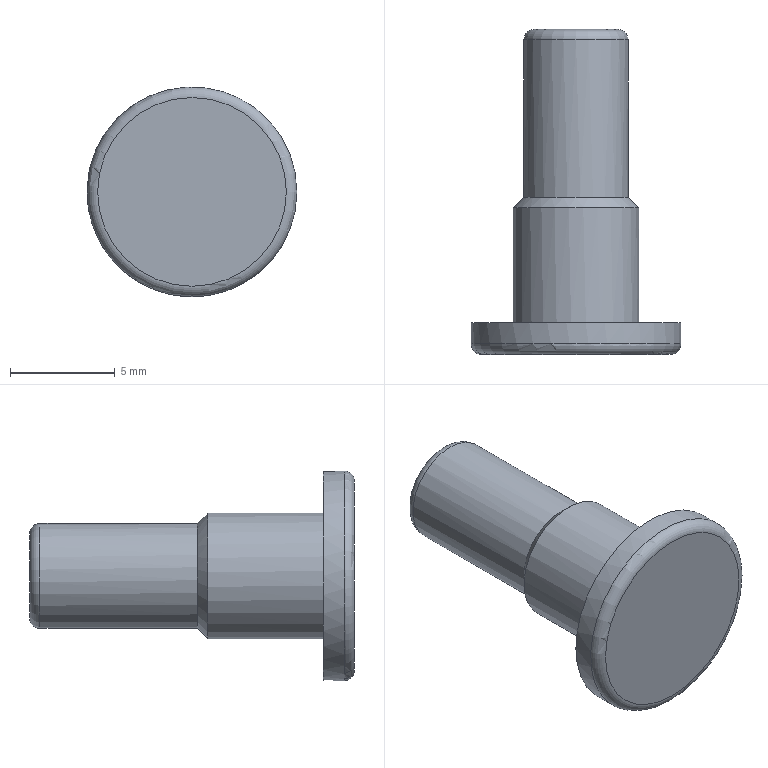Part | NX | features DATUM_CSYS 4, EXTRUDE 3, SKETCH 3, BLEND 2, CHAMFER 1 | 3 solids | 12 faces | box 10 x 15.5 x 10 mm | volume 439.857 mm3 | plane 6 | cylinder 3 | torus 2 | cone 1 | commonest cylinder face diameters 5 x1 6 x1 10 x1
STEP:
#1=CARTESIAN_POINT('',(0.,-1.,-5.));
#2=VERTEX_POINT('',#1);
#3=CARTESIAN_POINT('',(0.,-1.,0.));
#4=DIRECTION('',(0.,-1.,0.));
#5=DIRECTION('',(0.,0.,-1.));
#6=AXIS2_PLACEMENT_3D('',#3,#4,#5);
#7=CIRCLE('',#6,5.);
#8=EDGE_CURVE('',#2,#2,#7,.F.);
#9=ORIENTED_EDGE('',*,*,#8,.T.);
#10=EDGE_LOOP('',(#9));
#11=FACE_BOUND('',#10,.T.);
#12=CARTESIAN_POINT('',(5.,0.,0.));
#13=VERTEX_POINT('',#12);
#14=CARTESIAN_POINT('',(0.,0.,0.));
#15=DIRECTION('',(0.,-1.,0.));
#16=DIRECTION('',(1.,0.,0.));
#17=AXIS2_PLACEMENT_3D('',#14,#15,#16);
#18=CIRCLE('',#17,5.);
#19=EDGE_CURVE('',#13,#13,#18,.T.);
#20=ORIENTED_EDGE('',*,*,#19,.T.);
#21=EDGE_LOOP('',(#20));
#22=FACE_BOUND('',#21,.T.);
#23=CARTESIAN_POINT('',(0.,-1.5,0.));
#24=DIRECTION('',(0.,1.,0.));
#25=DIRECTION('',(0.,0.,1.));
#26=AXIS2_PLACEMENT_3D('',#23,#24,#25);
#27=CYLINDRICAL_SURFACE('',#26,5.);
#28=ADVANCED_FACE('',(#11,#22),#27,.T.);
#29=CARTESIAN_POINT('',(0.,-1.5,-4.5));
#30=VERTEX_POINT('',#29);
#31=CARTESIAN_POINT('',(0.,-1.5,0.));
#32=DIRECTION('',(0.,-1.,0.));
#33=DIRECTION('',(0.,0.,-1.));
#34=AXIS2_PLACEMENT_3D('',#31,#32,#33);
#35=CIRCLE('',#34,4.5);
#36=EDGE_CURVE('',#30,#30,#35,.T.);
#37=ORIENTED_EDGE('',*,*,#36,.T.);
#38=EDGE_LOOP('',(#37));
#39=FACE_BOUND('',#38,.T.);
#40=CARTESIAN_POINT('',(0.,-1.5,0.));
#41=DIRECTION('',(0.,-1.,0.));
#42=DIRECTION('',(0.,0.,-1.));
#43=AXIS2_PLACEMENT_3D('',#40,#41,#42);
#44=PLANE('',#43);
#45=ADVANCED_FACE('',(#39),#44,.T.);
#46=ORIENTED_EDGE('',*,*,#19,.F.);
#47=EDGE_LOOP('',(#46));
#48=FACE_BOUND('',#47,.T.);
#49=CARTESIAN_POINT('',(0.,0.,0.));
#50=DIRECTION('',(0.,-1.,0.));
#51=DIRECTION('',(0.,0.,-1.));
#52=AXIS2_PLACEMENT_3D('',#49,#50,#51);
#53=PLANE('',#52);
#54=ADVANCED_FACE('',(#48),#53,.F.);
#55=ORIENTED_EDGE('',*,*,#8,.F.);
#56=EDGE_LOOP('',(#55));
#57=FACE_BOUND('',#56,.T.);
#58=ORIENTED_EDGE('',*,*,#36,.F.);
#59=EDGE_LOOP('',(#58));
#60=FACE_BOUND('',#59,.T.);
#61=CARTESIAN_POINT('',(0.,-1.,0.));
#62=DIRECTION('',(0.,-1.,0.));
#63=DIRECTION('',(0.,0.,-1.));
#64=AXIS2_PLACEMENT_3D('',#61,#62,#63);
#65=TOROIDAL_SURFACE('',#64,4.5,0.5);
#66=ADVANCED_FACE('',(#57,#60),#65,.T.);
#67=CLOSED_SHELL('',(#28,#45,#54,#66));
#68=MANIFOLD_SOLID_BREP('',#67);
#69=CARTESIAN_POINT('',(0.,13.5,-2.5));
#70=VERTEX_POINT('',#69);
#71=CARTESIAN_POINT('',(0.,13.5,0.));
#72=DIRECTION('',(0.,-1.,0.));
#73=DIRECTION('',(0.,0.,-1.));
#74=AXIS2_PLACEMENT_3D('',#71,#72,#73);
#75=CIRCLE('',#74,2.5);
#76=EDGE_CURVE('',#70,#70,#75,.T.);
#77=ORIENTED_EDGE('',*,*,#76,.T.);
#78=EDGE_LOOP('',(#77));
#79=FACE_BOUND('',#78,.T.);
#80=CARTESIAN_POINT('',(2.5,6.,0.));
#81=VERTEX_POINT('',#80);
#82=CARTESIAN_POINT('',(0.,6.,0.));
#83=DIRECTION('',(0.,-1.,0.));
#84=DIRECTION('',(1.,0.,0.));
#85=AXIS2_PLACEMENT_3D('',#82,#83,#84);
#86=CIRCLE('',#85,2.5);
#87=EDGE_CURVE('',#81,#81,#86,.T.);
#88=ORIENTED_EDGE('',*,*,#87,.F.);
#89=EDGE_LOOP('',(#88));
#90=FACE_BOUND('',#89,.T.);
#91=CARTESIAN_POINT('',(0.,14.,0.));
#92=DIRECTION('',(0.,-1.,0.));
#93=DIRECTION('',(0.,0.,-1.));
#94=AXIS2_PLACEMENT_3D('',#91,#92,#93);
#95=CYLINDRICAL_SURFACE('',#94,2.5);
#96=ADVANCED_FACE('',(#79,#90),#95,.T.);
#97=CARTESIAN_POINT('',(0.,14.,-2.));
#98=VERTEX_POINT('',#97);
#99=CARTESIAN_POINT('',(0.,14.,0.));
#100=DIRECTION('',(0.,-1.,0.));
#101=DIRECTION('',(0.,0.,-1.));
#102=AXIS2_PLACEMENT_3D('',#99,#100,#101);
#103=CIRCLE('',#102,2.);
#104=EDGE_CURVE('',#98,#98,#103,.F.);
#105=ORIENTED_EDGE('',*,*,#104,.T.);
#106=EDGE_LOOP('',(#105));
#107=FACE_BOUND('',#106,.T.);
#108=CARTESIAN_POINT('',(0.,14.,0.));
#109=DIRECTION('',(0.,-1.,0.));
#110=DIRECTION('',(0.,0.,-1.));
#111=AXIS2_PLACEMENT_3D('',#108,#109,#110);
#112=PLANE('',#111);
#113=ADVANCED_FACE('',(#107),#112,.F.);
#114=ORIENTED_EDGE('',*,*,#87,.T.);
#115=EDGE_LOOP('',(#114));
#116=FACE_BOUND('',#115,.T.);
#117=CARTESIAN_POINT('',(0.,6.,0.));
#118=DIRECTION('',(0.,-1.,0.));
#119=DIRECTION('',(0.,0.,-1.));
#120=AXIS2_PLACEMENT_3D('',#117,#118,#119);
#121=PLANE('',#120);
#122=ADVANCED_FACE('',(#116),#121,.T.);
#123=ORIENTED_EDGE('',*,*,#104,.F.);
#124=EDGE_LOOP('',(#123));
#125=FACE_BOUND('',#124,.T.);
#126=ORIENTED_EDGE('',*,*,#76,.F.);
#127=EDGE_LOOP('',(#126));
#128=FACE_BOUND('',#127,.T.);
#129=CARTESIAN_POINT('',(0.,13.5,0.));
#130=DIRECTION('',(0.,-1.,0.));
#131=DIRECTION('',(0.,0.,-1.));
#132=AXIS2_PLACEMENT_3D('',#129,#130,#131);
#133=TOROIDAL_SURFACE('',#132,2.,0.5);
#134=ADVANCED_FACE('',(#125,#128),#133,.T.);
#135=CLOSED_SHELL('',(#96,#113,#122,#134));
#136=MANIFOLD_SOLID_BREP('',#135);
#137=CARTESIAN_POINT('',(0.,5.5,-3.));
#138=VERTEX_POINT('',#137);
#139=CARTESIAN_POINT('',(0.,5.5,0.));
#140=DIRECTION('',(0.,-1.,0.));
#141=DIRECTION('',(0.,0.,-1.));
#142=AXIS2_PLACEMENT_3D('',#139,#140,#141);
#143=CIRCLE('',#142,3.);
#144=EDGE_CURVE('',#138,#138,#143,.T.);
#145=ORIENTED_EDGE('',*,*,#144,.T.);
#146=EDGE_LOOP('',(#145));
#147=FACE_BOUND('',#146,.T.);
#148=CARTESIAN_POINT('',(3.,0.,0.));
#149=VERTEX_POINT('',#148);
#150=CARTESIAN_POINT('',(0.,0.,0.));
#151=DIRECTION('',(0.,-1.,0.));
#152=DIRECTION('',(1.,0.,0.));
#153=AXIS2_PLACEMENT_3D('',#150,#151,#152);
#154=CIRCLE('',#153,3.);
#155=EDGE_CURVE('',#149,#149,#154,.T.);
#156=ORIENTED_EDGE('',*,*,#155,.F.);
#157=EDGE_LOOP('',(#156));
#158=FACE_BOUND('',#157,.T.);
#159=CARTESIAN_POINT('',(0.,6.,0.));
#160=DIRECTION('',(0.,-1.,0.));
#161=DIRECTION('',(0.,0.,-1.));
#162=AXIS2_PLACEMENT_3D('',#159,#160,#161);
#163=CYLINDRICAL_SURFACE('',#162,3.);
#164=ADVANCED_FACE('',(#147,#158),#163,.T.);
#165=CARTESIAN_POINT('',(0.,6.,-2.5));
#166=VERTEX_POINT('',#165);
#167=CARTESIAN_POINT('',(0.,6.,0.));
#168=DIRECTION('',(0.,-1.,0.));
#169=DIRECTION('',(0.,0.,-1.));
#170=AXIS2_PLACEMENT_3D('',#167,#168,#169);
#171=CIRCLE('',#170,2.5);
#172=EDGE_CURVE('',#166,#166,#171,.F.);
#173=ORIENTED_EDGE('',*,*,#172,.T.);
#174=EDGE_LOOP('',(#173));
#175=FACE_BOUND('',#174,.T.);
#176=CARTESIAN_POINT('',(0.,6.,0.));
#177=DIRECTION('',(0.,-1.,0.));
#178=DIRECTION('',(0.,0.,-1.));
#179=AXIS2_PLACEMENT_3D('',#176,#177,#178);
#180=PLANE('',#179);
#181=ADVANCED_FACE('',(#175),#180,.F.);
#182=ORIENTED_EDGE('',*,*,#155,.T.);
#183=EDGE_LOOP('',(#182));
#184=FACE_BOUND('',#183,.T.);
#185=CARTESIAN_POINT('',(0.,0.,0.));
#186=DIRECTION('',(0.,-1.,0.));
#187=DIRECTION('',(0.,0.,-1.));
#188=AXIS2_PLACEMENT_3D('',#185,#186,#187);
#189=PLANE('',#188);
#190=ADVANCED_FACE('',(#184),#189,.T.);
#191=ORIENTED_EDGE('',*,*,#172,.F.);
#192=EDGE_LOOP('',(#191));
#193=FACE_BOUND('',#192,.T.);
#194=ORIENTED_EDGE('',*,*,#144,.F.);
#195=EDGE_LOOP('',(#194));
#196=FACE_BOUND('',#195,.T.);
#197=CARTESIAN_POINT('',(0.,5.5,0.));
#198=DIRECTION('',(0.,-1.,0.));
#199=DIRECTION('',(0.,0.,-1.));
#200=AXIS2_PLACEMENT_3D('',#197,#198,#199);
#201=CONICAL_SURFACE('',#200,3.,0.7854);
#202=ADVANCED_FACE('',(#193,#196),#201,.T.);
#203=CLOSED_SHELL('',(#164,#181,#190,#202));
#204=MANIFOLD_SOLID_BREP('',#203);
#205=(LENGTH_UNIT()NAMED_UNIT(*)SI_UNIT(.MILLI.,.METRE.));
#206=UNCERTAINTY_MEASURE_WITH_UNIT(LENGTH_MEASURE(0.00001),#205,'','');
#207=(NAMED_UNIT(*)PLANE_ANGLE_UNIT()SI_UNIT($,.RADIAN.));
#208=(NAMED_UNIT(*)SI_UNIT($,.STERADIAN.)SOLID_ANGLE_UNIT());
#209=(GEOMETRIC_REPRESENTATION_CONTEXT(3)GLOBAL_UNCERTAINTY_ASSIGNED_CONTEXT((#206))GLOBAL_UNIT_ASSIGNED_CONTEXT((#205,#207,#208))REPRESENTATION_CONTEXT('',''));
#210=ADVANCED_BREP_SHAPE_REPRESENTATION('',(#68,#136,#204),#209);